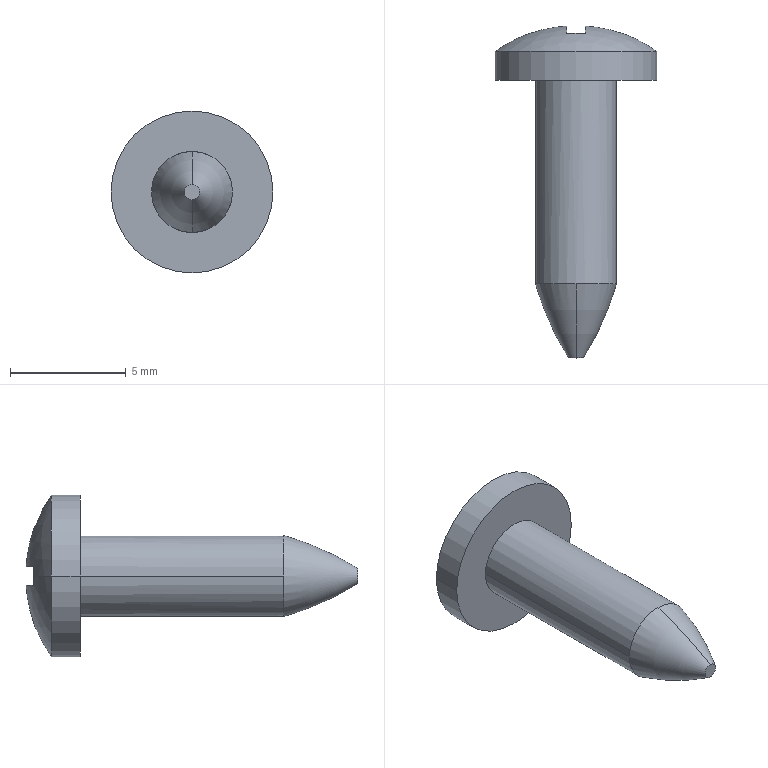Part | SolidWorks | features ICE 2, Revolution 2, CirPattern 1 | 1 solid | 23 faces | box 7 x 14.345 x 7 mm | volume 163.247 mm3 | plane 15 | cylinder 4 | torus 2 | sphere 2 | commonest cylinder face diameters 3.5 x2 7 x2
STEP:
#1=CARTESIAN_POINT('',(0.,-8.14,0.3269));
#2=VERTEX_POINT('',#1);
#3=CARTESIAN_POINT('',(0.,-8.14,-0.3269));
#4=VERTEX_POINT('',#3);
#5=CARTESIAN_POINT('',(0.,-8.14,0.));
#6=DIRECTION('',(0.,1.,0.));
#7=DIRECTION('',(0.,0.,1.));
#8=AXIS2_PLACEMENT_3D('',#5,#6,#7);
#9=CIRCLE('',#8,0.3269);
#10=EDGE_CURVE('',#2,#4,#9,.T.);
#11=ORIENTED_EDGE('',*,*,#10,.T.);
#12=CARTESIAN_POINT('',(0.,-4.94,-1.75));
#13=VERTEX_POINT('',#12);
#14=CARTESIAN_POINT('',(0.,-1.388,10.547));
#15=DIRECTION('',(1.,0.,0.));
#16=DIRECTION('',(0.,0.,-1.));
#17=AXIS2_PLACEMENT_3D('',#14,#15,#16);
#18=CIRCLE('',#17,12.8);
#19=EDGE_CURVE('',#4,#13,#18,.T.);
#20=ORIENTED_EDGE('',*,*,#19,.T.);
#21=CARTESIAN_POINT('',(1.75,-4.94,0.));
#22=VERTEX_POINT('',#21);
#23=CARTESIAN_POINT('',(0.,-4.94,0.));
#24=DIRECTION('',(0.,-1.,0.));
#25=DIRECTION('',(1.,0.,0.));
#26=AXIS2_PLACEMENT_3D('',#23,#24,#25);
#27=CIRCLE('',#26,1.75);
#28=EDGE_CURVE('',#13,#22,#27,.T.);
#29=ORIENTED_EDGE('',*,*,#28,.T.);
#30=CARTESIAN_POINT('',(0.,-4.94,1.75));
#31=VERTEX_POINT('',#30);
#32=CARTESIAN_POINT('',(0.,-4.94,0.));
#33=DIRECTION('',(0.,-1.,0.));
#34=DIRECTION('',(1.,0.,0.));
#35=AXIS2_PLACEMENT_3D('',#32,#33,#34);
#36=CIRCLE('',#35,1.75);
#37=EDGE_CURVE('',#22,#31,#36,.T.);
#38=ORIENTED_EDGE('',*,*,#37,.T.);
#39=CARTESIAN_POINT('',(0.,-1.388,-10.547));
#40=DIRECTION('',(-1.,0.,0.));
#41=DIRECTION('',(0.,0.,1.));
#42=AXIS2_PLACEMENT_3D('',#39,#40,#41);
#43=CIRCLE('',#42,12.8);
#44=EDGE_CURVE('',#2,#31,#43,.T.);
#45=ORIENTED_EDGE('',*,*,#44,.F.);
#46=EDGE_LOOP('',(#11,#20,#29,#38,#45));
#47=FACE_OUTER_BOUND('',#46,.T.);
#48=CARTESIAN_POINT('',(0.,-1.388,0.));
#49=DIRECTION('',(0.,1.,0.));
#50=DIRECTION('',(0.,0.,1.));
#51=AXIS2_PLACEMENT_3D('',#48,#49,#50);
#52=TOROIDAL_SURFACE('',#51,-10.547,12.8);
#53=ADVANCED_FACE('',(#47),#52,.T.);
#54=ORIENTED_EDGE('',*,*,#37,.F.);
#55=CARTESIAN_POINT('',(1.75,3.86,0.));
#56=VERTEX_POINT('',#55);
#57=CARTESIAN_POINT('',(1.75,-4.94,0.));
#58=DIRECTION('',(0.,1.,0.));
#59=VECTOR('',#58,1000.);
#60=LINE('',#57,#59);
#61=EDGE_CURVE('',#22,#56,#60,.T.);
#62=ORIENTED_EDGE('',*,*,#61,.T.);
#63=CARTESIAN_POINT('',(-1.75,3.86,0.));
#64=VERTEX_POINT('',#63);
#65=CARTESIAN_POINT('',(0.,3.86,0.));
#66=DIRECTION('',(0.,-1.,0.));
#67=DIRECTION('',(1.,0.,0.));
#68=AXIS2_PLACEMENT_3D('',#65,#66,#67);
#69=CIRCLE('',#68,1.75);
#70=EDGE_CURVE('',#56,#64,#69,.T.);
#71=ORIENTED_EDGE('',*,*,#70,.T.);
#72=CARTESIAN_POINT('',(-1.75,-4.94,0.));
#73=VERTEX_POINT('',#72);
#74=CARTESIAN_POINT('',(-1.75,-4.94,0.));
#75=DIRECTION('',(0.,1.,0.));
#76=VECTOR('',#75,1000.);
#77=LINE('',#74,#76);
#78=EDGE_CURVE('',#73,#64,#77,.T.);
#79=ORIENTED_EDGE('',*,*,#78,.F.);
#80=CARTESIAN_POINT('',(0.,-4.94,0.));
#81=DIRECTION('',(0.,-1.,0.));
#82=DIRECTION('',(1.,0.,0.));
#83=AXIS2_PLACEMENT_3D('',#80,#81,#82);
#84=CIRCLE('',#83,1.75);
#85=EDGE_CURVE('',#31,#73,#84,.T.);
#86=ORIENTED_EDGE('',*,*,#85,.F.);
#87=EDGE_LOOP('',(#54,#62,#71,#79,#86));
#88=FACE_OUTER_BOUND('',#87,.T.);
#89=CARTESIAN_POINT('',(0.,-4.94,0.));
#90=DIRECTION('',(0.,1.,0.));
#91=DIRECTION('',(-1.,0.,0.));
#92=AXIS2_PLACEMENT_3D('',#89,#90,#91);
#93=CYLINDRICAL_SURFACE('',#92,1.75);
#94=ADVANCED_FACE('',(#88),#93,.T.);
#95=CARTESIAN_POINT('',(-3.5,3.86,0.));
#96=VERTEX_POINT('',#95);
#97=CARTESIAN_POINT('',(3.5,3.86,0.));
#98=VERTEX_POINT('',#97);
#99=CARTESIAN_POINT('',(0.,3.86,0.));
#100=DIRECTION('',(0.,1.,0.));
#101=DIRECTION('',(-1.,0.,0.));
#102=AXIS2_PLACEMENT_3D('',#99,#100,#101);
#103=CIRCLE('',#102,3.5);
#104=EDGE_CURVE('',#96,#98,#103,.T.);
#105=ORIENTED_EDGE('',*,*,#104,.T.);
#106=CARTESIAN_POINT('',(3.5,5.105,0.));
#107=VERTEX_POINT('',#106);
#108=CARTESIAN_POINT('',(3.5,9.919,0.));
#109=DIRECTION('',(0.,1.,0.));
#110=VECTOR('',#109,1000.);
#111=LINE('',#108,#110);
#112=EDGE_CURVE('',#98,#107,#111,.T.);
#113=ORIENTED_EDGE('',*,*,#112,.T.);
#114=CARTESIAN_POINT('',(-3.5,5.105,0.));
#115=VERTEX_POINT('',#114);
#116=CARTESIAN_POINT('',(0.,5.105,0.));
#117=DIRECTION('',(0.,1.,0.));
#118=DIRECTION('',(-1.,0.,0.));
#119=AXIS2_PLACEMENT_3D('',#116,#117,#118);
#120=CIRCLE('',#119,3.5);
#121=EDGE_CURVE('',#115,#107,#120,.T.);
#122=ORIENTED_EDGE('',*,*,#121,.F.);
#123=CARTESIAN_POINT('',(-3.5,9.919,0.));
#124=DIRECTION('',(0.,1.,0.));
#125=VECTOR('',#124,1000.);
#126=LINE('',#123,#125);
#127=EDGE_CURVE('',#96,#115,#126,.T.);
#128=ORIENTED_EDGE('',*,*,#127,.F.);
#129=EDGE_LOOP('',(#105,#113,#122,#128));
#130=FACE_OUTER_BOUND('',#129,.T.);
#131=CARTESIAN_POINT('',(0.,9.919,0.));
#132=DIRECTION('',(0.,1.,0.));
#133=DIRECTION('',(-1.,0.,0.));
#134=AXIS2_PLACEMENT_3D('',#131,#132,#133);
#135=CYLINDRICAL_SURFACE('',#134,3.5);
#136=ADVANCED_FACE('',(#130),#135,.T.);
#137=CARTESIAN_POINT('',(0.,5.105,0.));
#138=DIRECTION('',(0.,1.,0.));
#139=DIRECTION('',(-1.,0.,0.));
#140=AXIS2_PLACEMENT_3D('',#137,#138,#139);
#141=CIRCLE('',#140,3.5);
#142=EDGE_CURVE('',#107,#115,#141,.T.);
#143=ORIENTED_EDGE('',*,*,#142,.T.);
#144=CARTESIAN_POINT('',(-2.,5.888,0.));
#145=VERTEX_POINT('',#144);
#146=CARTESIAN_POINT('',(0.,0.2313,0.));
#147=DIRECTION('',(0.,0.,-1.));
#148=DIRECTION('',(-1.,0.,0.));
#149=AXIS2_PLACEMENT_3D('',#146,#147,#148);
#150=CIRCLE('',#149,6.);
#151=EDGE_CURVE('',#115,#145,#150,.T.);
#152=ORIENTED_EDGE('',*,*,#151,.T.);
#153=CARTESIAN_POINT('',(-1.989,5.878,-0.4));
#154=VERTEX_POINT('',#153);
#155=CARTESIAN_POINT('',(1.855,2.137,0.));
#156=DIRECTION('',(-0.6974,-0.7167,0.));
#157=DIRECTION('',(0.7167,-0.6974,0.));
#158=AXIS2_PLACEMENT_3D('',#155,#156,#157);
#159=CIRCLE('',#158,5.378);
#160=EDGE_CURVE('',#145,#154,#159,.T.);
#161=ORIENTED_EDGE('',*,*,#160,.T.);
#162=CARTESIAN_POINT('',(-0.4,6.205,-0.4));
#163=VERTEX_POINT('',#162);
#164=CARTESIAN_POINT('',(0.,0.2313,-0.4));
#165=DIRECTION('',(0.,0.,1.));
#166=DIRECTION('',(1.,0.,0.));
#167=AXIS2_PLACEMENT_3D('',#164,#165,#166);
#168=CIRCLE('',#167,5.987);
#169=EDGE_CURVE('',#163,#154,#168,.T.);
#170=ORIENTED_EDGE('',*,*,#169,.F.);
#171=CARTESIAN_POINT('',(-0.4,5.878,-1.989));
#172=VERTEX_POINT('',#171);
#173=CARTESIAN_POINT('',(-0.4,0.2313,0.));
#174=DIRECTION('',(1.,0.,0.));
#175=DIRECTION('',(0.,0.,-1.));
#176=AXIS2_PLACEMENT_3D('',#173,#174,#175);
#177=CIRCLE('',#176,5.987);
#178=EDGE_CURVE('',#172,#163,#177,.T.);
#179=ORIENTED_EDGE('',*,*,#178,.F.);
#180=CARTESIAN_POINT('',(0.4,5.878,-1.989));
#181=VERTEX_POINT('',#180);
#182=CARTESIAN_POINT('',(0.,2.137,1.855));
#183=DIRECTION('',(0.,-0.7167,-0.6974));
#184=DIRECTION('',(0.,0.6974,-0.7167));
#185=AXIS2_PLACEMENT_3D('',#182,#183,#184);
#186=CIRCLE('',#185,5.378);
#187=EDGE_CURVE('',#172,#181,#186,.T.);
#188=ORIENTED_EDGE('',*,*,#187,.T.);
#189=CARTESIAN_POINT('',(0.4,6.205,-0.4));
#190=VERTEX_POINT('',#189);
#191=CARTESIAN_POINT('',(0.4,0.2313,0.));
#192=DIRECTION('',(1.,0.,0.));
#193=DIRECTION('',(0.,0.,-1.));
#194=AXIS2_PLACEMENT_3D('',#191,#192,#193);
#195=CIRCLE('',#194,5.987);
#196=EDGE_CURVE('',#181,#190,#195,.T.);
#197=ORIENTED_EDGE('',*,*,#196,.T.);
#198=CARTESIAN_POINT('',(1.989,5.878,-0.4));
#199=VERTEX_POINT('',#198);
#200=CARTESIAN_POINT('',(0.,0.2313,-0.4));
#201=DIRECTION('',(0.,0.,1.));
#202=DIRECTION('',(1.,0.,0.));
#203=AXIS2_PLACEMENT_3D('',#200,#201,#202);
#204=CIRCLE('',#203,5.987);
#205=EDGE_CURVE('',#199,#190,#204,.T.);
#206=ORIENTED_EDGE('',*,*,#205,.F.);
#207=CARTESIAN_POINT('',(2.,5.888,0.));
#208=VERTEX_POINT('',#207);
#209=CARTESIAN_POINT('',(-1.855,2.137,0.));
#210=DIRECTION('',(0.6974,-0.7167,0.));
#211=DIRECTION('',(0.7167,0.6974,0.));
#212=AXIS2_PLACEMENT_3D('',#209,#210,#211);
#213=CIRCLE('',#212,5.378);
#214=EDGE_CURVE('',#199,#208,#213,.T.);
#215=ORIENTED_EDGE('',*,*,#214,.T.);
#216=CARTESIAN_POINT('',(0.,0.2313,0.));
#217=DIRECTION('',(0.,0.,1.));
#218=DIRECTION('',(1.,0.,0.));
#219=AXIS2_PLACEMENT_3D('',#216,#217,#218);
#220=CIRCLE('',#219,6.);
#221=EDGE_CURVE('',#107,#208,#220,.T.);
#222=ORIENTED_EDGE('',*,*,#221,.F.);
#223=EDGE_LOOP('',(#143,#152,#161,#170,#179,#188,#197,#206,#215,#222));
#224=FACE_OUTER_BOUND('',#223,.T.);
#225=CARTESIAN_POINT('',(0.,0.2313,0.));
#226=DIRECTION('',(0.,0.,-1.));
#227=DIRECTION('',(1.,0.,0.));
#228=AXIS2_PLACEMENT_3D('',#225,#226,#227);
#229=SPHERICAL_SURFACE('',#228,6.);
#230=ADVANCED_FACE('',(#224),#229,.T.);
#231=ORIENTED_EDGE('',*,*,#151,.F.);
#232=ORIENTED_EDGE('',*,*,#121,.T.);
#233=ORIENTED_EDGE('',*,*,#221,.T.);
#234=CARTESIAN_POINT('',(1.989,5.878,0.4));
#235=VERTEX_POINT('',#234);
#236=CARTESIAN_POINT('',(-1.855,2.137,0.));
#237=DIRECTION('',(0.6974,-0.7167,0.));
#238=DIRECTION('',(0.7167,0.6974,0.));
#239=AXIS2_PLACEMENT_3D('',#236,#237,#238);
#240=CIRCLE('',#239,5.378);
#241=EDGE_CURVE('',#208,#235,#240,.T.);
#242=ORIENTED_EDGE('',*,*,#241,.T.);
#243=CARTESIAN_POINT('',(0.4,6.205,0.4));
#244=VERTEX_POINT('',#243);
#245=CARTESIAN_POINT('',(0.,0.2313,0.4));
#246=DIRECTION('',(0.,0.,1.));
#247=DIRECTION('',(1.,0.,0.));
#248=AXIS2_PLACEMENT_3D('',#245,#246,#247);
#249=CIRCLE('',#248,5.987);
#250=EDGE_CURVE('',#235,#244,#249,.T.);
#251=ORIENTED_EDGE('',*,*,#250,.T.);
#252=CARTESIAN_POINT('',(0.4,5.878,1.989));
#253=VERTEX_POINT('',#252);
#254=CARTESIAN_POINT('',(0.4,0.2313,0.));
#255=DIRECTION('',(1.,0.,0.));
#256=DIRECTION('',(0.,0.,-1.));
#257=AXIS2_PLACEMENT_3D('',#254,#255,#256);
#258=CIRCLE('',#257,5.987);
#259=EDGE_CURVE('',#244,#253,#258,.T.);
#260=ORIENTED_EDGE('',*,*,#259,.T.);
#261=CARTESIAN_POINT('',(-0.4,5.878,1.989));
#262=VERTEX_POINT('',#261);
#263=CARTESIAN_POINT('',(0.,2.137,-1.855));
#264=DIRECTION('',(0.,-0.7167,0.6974));
#265=DIRECTION('',(0.,-0.6974,-0.7167));
#266=AXIS2_PLACEMENT_3D('',#263,#264,#265);
#267=CIRCLE('',#266,5.378);
#268=EDGE_CURVE('',#253,#262,#267,.T.);
#269=ORIENTED_EDGE('',*,*,#268,.T.);
#270=CARTESIAN_POINT('',(-0.4,6.205,0.4));
#271=VERTEX_POINT('',#270);
#272=CARTESIAN_POINT('',(-0.4,0.2313,0.));
#273=DIRECTION('',(1.,0.,0.));
#274=DIRECTION('',(0.,0.,-1.));
#275=AXIS2_PLACEMENT_3D('',#272,#273,#274);
#276=CIRCLE('',#275,5.987);
#277=EDGE_CURVE('',#271,#262,#276,.T.);
#278=ORIENTED_EDGE('',*,*,#277,.F.);
#279=CARTESIAN_POINT('',(-1.989,5.878,0.4));
#280=VERTEX_POINT('',#279);
#281=CARTESIAN_POINT('',(0.,0.2313,0.4));
#282=DIRECTION('',(0.,0.,1.));
#283=DIRECTION('',(1.,0.,0.));
#284=AXIS2_PLACEMENT_3D('',#281,#282,#283);
#285=CIRCLE('',#284,5.987);
#286=EDGE_CURVE('',#271,#280,#285,.T.);
#287=ORIENTED_EDGE('',*,*,#286,.T.);
#288=CARTESIAN_POINT('',(1.855,2.137,0.));
#289=DIRECTION('',(-0.6974,-0.7167,0.));
#290=DIRECTION('',(0.7167,-0.6974,0.));
#291=AXIS2_PLACEMENT_3D('',#288,#289,#290);
#292=CIRCLE('',#291,5.378);
#293=EDGE_CURVE('',#280,#145,#292,.T.);
#294=ORIENTED_EDGE('',*,*,#293,.T.);
#295=EDGE_LOOP('',(#231,#232,#233,#242,#251,#260,#269,#278,#287,#294));
#296=FACE_OUTER_BOUND('',#295,.T.);
#297=CARTESIAN_POINT('',(0.,0.2313,0.));
#298=DIRECTION('',(0.,0.,-1.));
#299=DIRECTION('',(1.,0.,0.));
#300=AXIS2_PLACEMENT_3D('',#297,#298,#299);
#301=SPHERICAL_SURFACE('',#300,6.);
#302=ADVANCED_FACE('',(#296),#301,.T.);
#303=CARTESIAN_POINT('',(-0.4,4.331,-0.4));
#304=VERTEX_POINT('',#303);
#305=CARTESIAN_POINT('',(-2.,5.888,-0.4));
#306=DIRECTION('',(0.7167,-0.6974,0.));
#307=VECTOR('',#306,1000.);
#308=LINE('',#305,#307);
#309=EDGE_CURVE('',#154,#304,#308,.T.);
#310=ORIENTED_EDGE('',*,*,#309,.T.);
#311=CARTESIAN_POINT('',(-0.4,0.2313,-0.4));
#312=DIRECTION('',(0.,1.,0.));
#313=VECTOR('',#312,1000.);
#314=LINE('',#311,#313);
#315=EDGE_CURVE('',#304,#163,#314,.T.);
#316=ORIENTED_EDGE('',*,*,#315,.T.);
#317=ORIENTED_EDGE('',*,*,#169,.T.);
#318=EDGE_LOOP('',(#310,#316,#317));
#319=FACE_OUTER_BOUND('',#318,.T.);
#320=CARTESIAN_POINT('',(0.,0.2313,-0.4));
#321=DIRECTION('',(0.,0.,1.));
#322=DIRECTION('',(1.,0.,0.));
#323=AXIS2_PLACEMENT_3D('',#320,#321,#322);
#324=PLANE('',#323);
#325=ADVANCED_FACE('',(#319),#324,.T.);
#326=CARTESIAN_POINT('',(-0.4,4.331,0.4));
#327=VERTEX_POINT('',#326);
#328=CARTESIAN_POINT('',(-0.4,0.2313,0.4));
#329=DIRECTION('',(0.,1.,0.));
#330=VECTOR('',#329,1000.);
#331=LINE('',#328,#330);
#332=EDGE_CURVE('',#327,#271,#331,.T.);
#333=ORIENTED_EDGE('',*,*,#332,.F.);
#334=CARTESIAN_POINT('',(-2.,5.888,0.4));
#335=DIRECTION('',(0.7167,-0.6974,0.));
#336=VECTOR('',#335,1000.);
#337=LINE('',#334,#336);
#338=EDGE_CURVE('',#280,#327,#337,.T.);
#339=ORIENTED_EDGE('',*,*,#338,.F.);
#340=ORIENTED_EDGE('',*,*,#286,.F.);
#341=EDGE_LOOP('',(#333,#339,#340));
#342=FACE_OUTER_BOUND('',#341,.T.);
#343=CARTESIAN_POINT('',(0.,0.2313,0.4));
#344=DIRECTION('',(0.,0.,1.));
#345=DIRECTION('',(1.,0.,0.));
#346=AXIS2_PLACEMENT_3D('',#343,#344,#345);
#347=PLANE('',#346);
#348=ADVANCED_FACE('',(#342),#347,.F.);
#349=CARTESIAN_POINT('',(0.,3.86,0.));
#350=DIRECTION('',(0.,-1.,0.));
#351=DIRECTION('',(1.,0.,0.));
#352=AXIS2_PLACEMENT_3D('',#349,#350,#351);
#353=CIRCLE('',#352,1.75);
#354=EDGE_CURVE('',#64,#56,#353,.T.);
#355=ORIENTED_EDGE('',*,*,#354,.F.);
#356=ORIENTED_EDGE('',*,*,#70,.F.);
#357=EDGE_LOOP('',(#355,#356));
#358=FACE_BOUND('',#357,.T.);
#359=ORIENTED_EDGE('',*,*,#104,.F.);
#360=CARTESIAN_POINT('',(0.,3.86,0.));
#361=DIRECTION('',(0.,1.,0.));
#362=DIRECTION('',(-1.,0.,0.));
#363=AXIS2_PLACEMENT_3D('',#360,#361,#362);
#364=CIRCLE('',#363,3.5);
#365=EDGE_CURVE('',#98,#96,#364,.T.);
#366=ORIENTED_EDGE('',*,*,#365,.F.);
#367=EDGE_LOOP('',(#359,#366));
#368=FACE_OUTER_BOUND('',#367,.T.);
#369=CARTESIAN_POINT('',(0.,3.86,0.));
#370=DIRECTION('',(0.,1.,0.));
#371=DIRECTION('',(-1.,0.,0.));
#372=AXIS2_PLACEMENT_3D('',#369,#370,#371);
#373=PLANE('',#372);
#374=ADVANCED_FACE('',(#358,#368),#373,.F.);
#375=ORIENTED_EDGE('',*,*,#112,.F.);
#376=ORIENTED_EDGE('',*,*,#365,.T.);
#377=ORIENTED_EDGE('',*,*,#127,.T.);
#378=ORIENTED_EDGE('',*,*,#142,.F.);
#379=EDGE_LOOP('',(#375,#376,#377,#378));
#380=FACE_OUTER_BOUND('',#379,.T.);
#381=CARTESIAN_POINT('',(0.,9.919,0.));
#382=DIRECTION('',(0.,1.,0.));
#383=DIRECTION('',(-1.,0.,0.));
#384=AXIS2_PLACEMENT_3D('',#381,#382,#383);
#385=CYLINDRICAL_SURFACE('',#384,3.5);
#386=ADVANCED_FACE('',(#380),#385,.T.);
#387=ORIENTED_EDGE('',*,*,#61,.F.);
#388=ORIENTED_EDGE('',*,*,#28,.F.);
#389=CARTESIAN_POINT('',(0.,-4.94,0.));
#390=DIRECTION('',(0.,-1.,0.));
#391=DIRECTION('',(1.,0.,0.));
#392=AXIS2_PLACEMENT_3D('',#389,#390,#391);
#393=CIRCLE('',#392,1.75);
#394=EDGE_CURVE('',#73,#13,#393,.T.);
#395=ORIENTED_EDGE('',*,*,#394,.F.);
#396=ORIENTED_EDGE('',*,*,#78,.T.);
#397=ORIENTED_EDGE('',*,*,#354,.T.);
#398=EDGE_LOOP('',(#387,#388,#395,#396,#397));
#399=FACE_OUTER_BOUND('',#398,.T.);
#400=CARTESIAN_POINT('',(0.,-4.94,0.));
#401=DIRECTION('',(0.,1.,0.));
#402=DIRECTION('',(-1.,0.,0.));
#403=AXIS2_PLACEMENT_3D('',#400,#401,#402);
#404=CYLINDRICAL_SURFACE('',#403,1.75);
#405=ADVANCED_FACE('',(#399),#404,.T.);
#406=ORIENTED_EDGE('',*,*,#19,.F.);
#407=CARTESIAN_POINT('',(0.,-8.14,0.));
#408=DIRECTION('',(0.,1.,0.));
#409=DIRECTION('',(0.,0.,1.));
#410=AXIS2_PLACEMENT_3D('',#407,#408,#409);
#411=CIRCLE('',#410,0.3269);
#412=EDGE_CURVE('',#4,#2,#411,.T.);
#413=ORIENTED_EDGE('',*,*,#412,.T.);
#414=ORIENTED_EDGE('',*,*,#44,.T.);
#415=ORIENTED_EDGE('',*,*,#85,.T.);
#416=ORIENTED_EDGE('',*,*,#394,.T.);
#417=EDGE_LOOP('',(#406,#413,#414,#415,#416));
#418=FACE_OUTER_BOUND('',#417,.T.);
#419=CARTESIAN_POINT('',(0.,-1.388,0.));
#420=DIRECTION('',(0.,1.,0.));
#421=DIRECTION('',(0.,0.,1.));
#422=AXIS2_PLACEMENT_3D('',#419,#420,#421);
#423=TOROIDAL_SURFACE('',#422,-10.547,12.8);
#424=ADVANCED_FACE('',(#418),#423,.T.);
#425=ORIENTED_EDGE('',*,*,#10,.F.);
#426=ORIENTED_EDGE('',*,*,#412,.F.);
#427=EDGE_LOOP('',(#425,#426));
#428=FACE_OUTER_BOUND('',#427,.T.);
#429=CARTESIAN_POINT('',(-0.3269,-8.14,0.));
#430=DIRECTION('',(0.,-1.,0.));
#431=DIRECTION('',(0.,0.,-1.));
#432=AXIS2_PLACEMENT_3D('',#429,#430,#431);
#433=PLANE('',#432);
#434=ADVANCED_FACE('',(#428),#433,.T.);
#435=ORIENTED_EDGE('',*,*,#214,.F.);
#436=CARTESIAN_POINT('',(0.4,4.331,-0.4));
#437=VERTEX_POINT('',#436);
#438=CARTESIAN_POINT('',(0.4,4.331,-0.4));
#439=DIRECTION('',(0.7167,0.6974,0.));
#440=VECTOR('',#439,1000.);
#441=LINE('',#438,#440);
#442=EDGE_CURVE('',#437,#199,#441,.T.);
#443=ORIENTED_EDGE('',*,*,#442,.F.);
#444=CARTESIAN_POINT('',(0.4,4.331,0.4));
#445=VERTEX_POINT('',#444);
#446=CARTESIAN_POINT('',(0.4,4.331,-0.4));
#447=DIRECTION('',(0.,0.,1.));
#448=VECTOR('',#447,1000.);
#449=LINE('',#446,#448);
#450=EDGE_CURVE('',#437,#445,#449,.T.);
#451=ORIENTED_EDGE('',*,*,#450,.T.);
#452=CARTESIAN_POINT('',(0.4,4.331,0.4));
#453=DIRECTION('',(0.7167,0.6974,0.));
#454=VECTOR('',#453,1000.);
#455=LINE('',#452,#454);
#456=EDGE_CURVE('',#445,#235,#455,.T.);
#457=ORIENTED_EDGE('',*,*,#456,.T.);
#458=ORIENTED_EDGE('',*,*,#241,.F.);
#459=EDGE_LOOP('',(#435,#443,#451,#457,#458));
#460=FACE_OUTER_BOUND('',#459,.T.);
#461=CARTESIAN_POINT('',(0.4,4.331,-0.4));
#462=DIRECTION('',(0.6974,-0.7167,0.));
#463=DIRECTION('',(0.7167,0.6974,0.));
#464=AXIS2_PLACEMENT_3D('',#461,#462,#463);
#465=PLANE('',#464);
#466=ADVANCED_FACE('',(#460),#465,.F.);
#467=ORIENTED_EDGE('',*,*,#338,.T.);
#468=CARTESIAN_POINT('',(-0.4,4.331,-0.4));
#469=DIRECTION('',(0.,0.,1.));
#470=VECTOR('',#469,1000.);
#471=LINE('',#468,#470);
#472=EDGE_CURVE('',#304,#327,#471,.T.);
#473=ORIENTED_EDGE('',*,*,#472,.F.);
#474=ORIENTED_EDGE('',*,*,#309,.F.);
#475=ORIENTED_EDGE('',*,*,#160,.F.);
#476=ORIENTED_EDGE('',*,*,#293,.F.);
#477=EDGE_LOOP('',(#467,#473,#474,#475,#476));
#478=FACE_OUTER_BOUND('',#477,.T.);
#479=CARTESIAN_POINT('',(-2.,5.888,-0.4));
#480=DIRECTION('',(-0.6974,-0.7167,0.));
#481=DIRECTION('',(0.7167,-0.6974,0.));
#482=AXIS2_PLACEMENT_3D('',#479,#480,#481);
#483=PLANE('',#482);
#484=ADVANCED_FACE('',(#478),#483,.F.);
#485=CARTESIAN_POINT('',(0.4,0.2313,-0.4));
#486=DIRECTION('',(0.,1.,0.));
#487=VECTOR('',#486,1000.);
#488=LINE('',#485,#487);
#489=EDGE_CURVE('',#437,#190,#488,.T.);
#490=ORIENTED_EDGE('',*,*,#489,.F.);
#491=ORIENTED_EDGE('',*,*,#442,.T.);
#492=ORIENTED_EDGE('',*,*,#205,.T.);
#493=EDGE_LOOP('',(#490,#491,#492));
#494=FACE_OUTER_BOUND('',#493,.T.);
#495=CARTESIAN_POINT('',(0.,0.2313,-0.4));
#496=DIRECTION('',(0.,0.,1.));
#497=DIRECTION('',(1.,0.,0.));
#498=AXIS2_PLACEMENT_3D('',#495,#496,#497);
#499=PLANE('',#498);
#500=ADVANCED_FACE('',(#494),#499,.T.);
#501=ORIENTED_EDGE('',*,*,#456,.F.);
#502=CARTESIAN_POINT('',(0.4,0.2313,0.4));
#503=DIRECTION('',(0.,1.,0.));
#504=VECTOR('',#503,1000.);
#505=LINE('',#502,#504);
#506=EDGE_CURVE('',#445,#244,#505,.T.);
#507=ORIENTED_EDGE('',*,*,#506,.T.);
#508=ORIENTED_EDGE('',*,*,#250,.F.);
#509=EDGE_LOOP('',(#501,#507,#508));
#510=FACE_OUTER_BOUND('',#509,.T.);
#511=CARTESIAN_POINT('',(0.,0.2313,0.4));
#512=DIRECTION('',(0.,0.,1.));
#513=DIRECTION('',(1.,0.,0.));
#514=AXIS2_PLACEMENT_3D('',#511,#512,#513);
#515=PLANE('',#514);
#516=ADVANCED_FACE('',(#510),#515,.F.);
#517=CARTESIAN_POINT('',(-0.4,4.331,0.4));
#518=DIRECTION('',(1.,0.,0.));
#519=VECTOR('',#518,1000.);
#520=LINE('',#517,#519);
#521=EDGE_CURVE('',#327,#445,#520,.T.);
#522=ORIENTED_EDGE('',*,*,#521,.T.);
#523=ORIENTED_EDGE('',*,*,#450,.F.);
#524=CARTESIAN_POINT('',(-0.4,4.331,-0.4));
#525=DIRECTION('',(1.,0.,0.));
#526=VECTOR('',#525,1000.);
#527=LINE('',#524,#526);
#528=EDGE_CURVE('',#304,#437,#527,.T.);
#529=ORIENTED_EDGE('',*,*,#528,.F.);
#530=ORIENTED_EDGE('',*,*,#472,.T.);
#531=EDGE_LOOP('',(#522,#523,#529,#530));
#532=FACE_OUTER_BOUND('',#531,.T.);
#533=CARTESIAN_POINT('',(-0.4,4.331,-0.4));
#534=DIRECTION('',(0.,-1.,0.));
#535=DIRECTION('',(1.,0.,0.));
#536=AXIS2_PLACEMENT_3D('',#533,#534,#535);
#537=PLANE('',#536);
#538=ADVANCED_FACE('',(#532),#537,.F.);
#539=CARTESIAN_POINT('',(0.4,5.888,2.));
#540=DIRECTION('',(0.,-0.6974,-0.7167));
#541=VECTOR('',#540,1000.);
#542=LINE('',#539,#541);
#543=EDGE_CURVE('',#253,#445,#542,.T.);
#544=ORIENTED_EDGE('',*,*,#543,.T.);
#545=ORIENTED_EDGE('',*,*,#521,.F.);
#546=CARTESIAN_POINT('',(-0.4,5.888,2.));
#547=DIRECTION('',(0.,-0.6974,-0.7167));
#548=VECTOR('',#547,1000.);
#549=LINE('',#546,#548);
#550=EDGE_CURVE('',#262,#327,#549,.T.);
#551=ORIENTED_EDGE('',*,*,#550,.F.);
#552=ORIENTED_EDGE('',*,*,#268,.F.);
#553=EDGE_LOOP('',(#544,#545,#551,#552));
#554=FACE_OUTER_BOUND('',#553,.T.);
#555=CARTESIAN_POINT('',(-0.4,5.888,2.));
#556=DIRECTION('',(0.,-0.7167,0.6974));
#557=DIRECTION('',(0.,-0.6974,-0.7167));
#558=AXIS2_PLACEMENT_3D('',#555,#556,#557);
#559=PLANE('',#558);
#560=ADVANCED_FACE('',(#554),#559,.F.);
#561=ORIENTED_EDGE('',*,*,#506,.F.);
#562=ORIENTED_EDGE('',*,*,#543,.F.);
#563=ORIENTED_EDGE('',*,*,#259,.F.);
#564=EDGE_LOOP('',(#561,#562,#563));
#565=FACE_OUTER_BOUND('',#564,.T.);
#566=CARTESIAN_POINT('',(0.4,0.2313,0.));
#567=DIRECTION('',(1.,0.,0.));
#568=DIRECTION('',(0.,0.,-1.));
#569=AXIS2_PLACEMENT_3D('',#566,#567,#568);
#570=PLANE('',#569);
#571=ADVANCED_FACE('',(#565),#570,.F.);
#572=ORIENTED_EDGE('',*,*,#277,.T.);
#573=ORIENTED_EDGE('',*,*,#550,.T.);
#574=ORIENTED_EDGE('',*,*,#332,.T.);
#575=EDGE_LOOP('',(#572,#573,#574));
#576=FACE_OUTER_BOUND('',#575,.T.);
#577=CARTESIAN_POINT('',(-0.4,0.2313,0.));
#578=DIRECTION('',(1.,0.,0.));
#579=DIRECTION('',(0.,0.,-1.));
#580=AXIS2_PLACEMENT_3D('',#577,#578,#579);
#581=PLANE('',#580);
#582=ADVANCED_FACE('',(#576),#581,.T.);
#583=ORIENTED_EDGE('',*,*,#187,.F.);
#584=CARTESIAN_POINT('',(-0.4,4.331,-0.4));
#585=DIRECTION('',(0.,0.6974,-0.7167));
#586=VECTOR('',#585,1000.);
#587=LINE('',#584,#586);
#588=EDGE_CURVE('',#304,#172,#587,.T.);
#589=ORIENTED_EDGE('',*,*,#588,.F.);
#590=ORIENTED_EDGE('',*,*,#528,.T.);
#591=CARTESIAN_POINT('',(0.4,4.331,-0.4));
#592=DIRECTION('',(0.,0.6974,-0.7167));
#593=VECTOR('',#592,1000.);
#594=LINE('',#591,#593);
#595=EDGE_CURVE('',#437,#181,#594,.T.);
#596=ORIENTED_EDGE('',*,*,#595,.T.);
#597=EDGE_LOOP('',(#583,#589,#590,#596));
#598=FACE_OUTER_BOUND('',#597,.T.);
#599=CARTESIAN_POINT('',(-0.4,4.331,-0.4));
#600=DIRECTION('',(0.,-0.7167,-0.6974));
#601=DIRECTION('',(0.,0.6974,-0.7167));
#602=AXIS2_PLACEMENT_3D('',#599,#600,#601);
#603=PLANE('',#602);
#604=ADVANCED_FACE('',(#598),#603,.F.);
#605=ORIENTED_EDGE('',*,*,#178,.T.);
#606=ORIENTED_EDGE('',*,*,#315,.F.);
#607=ORIENTED_EDGE('',*,*,#588,.T.);
#608=EDGE_LOOP('',(#605,#606,#607));
#609=FACE_OUTER_BOUND('',#608,.T.);
#610=CARTESIAN_POINT('',(-0.4,0.2313,0.));
#611=DIRECTION('',(1.,0.,0.));
#612=DIRECTION('',(0.,0.,-1.));
#613=AXIS2_PLACEMENT_3D('',#610,#611,#612);
#614=PLANE('',#613);
#615=ADVANCED_FACE('',(#609),#614,.T.);
#616=ORIENTED_EDGE('',*,*,#595,.F.);
#617=ORIENTED_EDGE('',*,*,#489,.T.);
#618=ORIENTED_EDGE('',*,*,#196,.F.);
#619=EDGE_LOOP('',(#616,#617,#618));
#620=FACE_OUTER_BOUND('',#619,.T.);
#621=CARTESIAN_POINT('',(0.4,0.2313,0.));
#622=DIRECTION('',(1.,0.,0.));
#623=DIRECTION('',(0.,0.,-1.));
#624=AXIS2_PLACEMENT_3D('',#621,#622,#623);
#625=PLANE('',#624);
#626=ADVANCED_FACE('',(#620),#625,.F.);
#627=CLOSED_SHELL('',(#53,#94,#136,#230,#302,#325,#348,#374,#386,#405,#424,#434,#466,#484,#500,#516,#538,#560,#571,#582,#604,#615,#626));
#628=MANIFOLD_SOLID_BREP('',#627);
#629=CARTESIAN_POINT('',(0.,0.,0.));
#630=DIRECTION('',(0.,0.,1.));
#631=DIRECTION('',(1.,0.,0.));
#632=AXIS2_PLACEMENT_3D('',#629,#630,#631);
#633=(LENGTH_UNIT()NAMED_UNIT(*)SI_UNIT(.MILLI.,.METRE.));
#634=UNCERTAINTY_MEASURE_WITH_UNIT(LENGTH_MEASURE(0.00001),#633,'','');
#635=(NAMED_UNIT(*)PLANE_ANGLE_UNIT()SI_UNIT($,.RADIAN.));
#636=(NAMED_UNIT(*)SI_UNIT($,.STERADIAN.)SOLID_ANGLE_UNIT());
#637=(GEOMETRIC_REPRESENTATION_CONTEXT(3)GLOBAL_UNCERTAINTY_ASSIGNED_CONTEXT((#634))GLOBAL_UNIT_ASSIGNED_CONTEXT((#633,#635,#636))REPRESENTATION_CONTEXT('',''));
#638=ADVANCED_BREP_SHAPE_REPRESENTATION('',(#628,#632),#637);